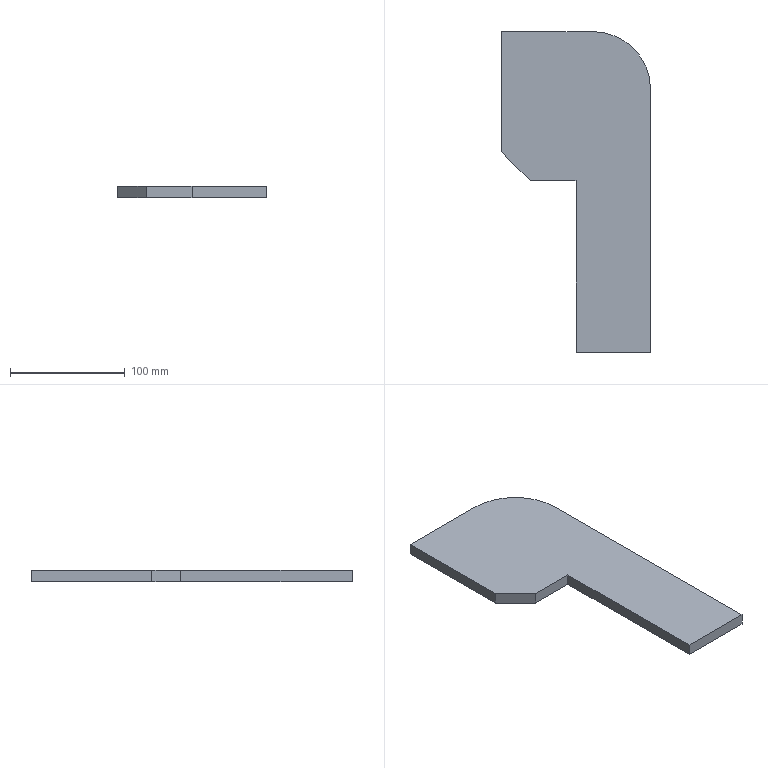Part | SolidWorks | features Extrusion 1 | 1 solid | 10 faces | box 130 x 280 x 10 mm | volume 258010 mm3 | plane 9 | cylinder 1 | commonest cylinder face diameters 100 x1
STEP:
#1=CARTESIAN_POINT('',(80.,280.,-5.));
#2=VERTEX_POINT('',#1);
#3=CARTESIAN_POINT('',(0.,280.,-5.));
#4=VERTEX_POINT('',#3);
#5=CARTESIAN_POINT('',(0.,280.,-5.));
#6=DIRECTION('',(-1.,0.,0.));
#7=VECTOR('',#6,1000.);
#8=LINE('',#5,#7);
#9=EDGE_CURVE('',#2,#4,#8,.T.);
#10=ORIENTED_EDGE('',*,*,#9,.T.);
#11=CARTESIAN_POINT('',(0.,280.,5.));
#12=VERTEX_POINT('',#11);
#13=CARTESIAN_POINT('',(0.,280.,5.));
#14=DIRECTION('',(0.,0.,-1.));
#15=VECTOR('',#14,1000.);
#16=LINE('',#13,#15);
#17=EDGE_CURVE('',#12,#4,#16,.T.);
#18=ORIENTED_EDGE('',*,*,#17,.F.);
#19=CARTESIAN_POINT('',(80.,280.,5.));
#20=VERTEX_POINT('',#19);
#21=CARTESIAN_POINT('',(0.,280.,5.));
#22=DIRECTION('',(-1.,0.,0.));
#23=VECTOR('',#22,1000.);
#24=LINE('',#21,#23);
#25=EDGE_CURVE('',#20,#12,#24,.T.);
#26=ORIENTED_EDGE('',*,*,#25,.F.);
#27=CARTESIAN_POINT('',(80.,280.,5.));
#28=DIRECTION('',(0.,0.,-1.));
#29=VECTOR('',#28,1000.);
#30=LINE('',#27,#29);
#31=EDGE_CURVE('',#20,#2,#30,.T.);
#32=ORIENTED_EDGE('',*,*,#31,.T.);
#33=EDGE_LOOP('',(#10,#18,#26,#32));
#34=FACE_OUTER_BOUND('',#33,.T.);
#35=CARTESIAN_POINT('',(0.,280.,5.));
#36=DIRECTION('',(0.,-1.,0.));
#37=DIRECTION('',(0.,0.,-1.));
#38=AXIS2_PLACEMENT_3D('',#35,#36,#37);
#39=PLANE('',#38);
#40=ADVANCED_FACE('',(#34),#39,.F.);
#41=CARTESIAN_POINT('',(0.,175.,-5.));
#42=VERTEX_POINT('',#41);
#43=CARTESIAN_POINT('',(0.,175.,-5.));
#44=DIRECTION('',(0.,-1.,0.));
#45=VECTOR('',#44,1000.);
#46=LINE('',#43,#45);
#47=EDGE_CURVE('',#4,#42,#46,.T.);
#48=ORIENTED_EDGE('',*,*,#47,.T.);
#49=CARTESIAN_POINT('',(0.,175.,5.));
#50=VERTEX_POINT('',#49);
#51=CARTESIAN_POINT('',(0.,175.,5.));
#52=DIRECTION('',(0.,0.,-1.));
#53=VECTOR('',#52,1000.);
#54=LINE('',#51,#53);
#55=EDGE_CURVE('',#50,#42,#54,.T.);
#56=ORIENTED_EDGE('',*,*,#55,.F.);
#57=CARTESIAN_POINT('',(0.,175.,5.));
#58=DIRECTION('',(0.,-1.,0.));
#59=VECTOR('',#58,1000.);
#60=LINE('',#57,#59);
#61=EDGE_CURVE('',#12,#50,#60,.T.);
#62=ORIENTED_EDGE('',*,*,#61,.F.);
#63=ORIENTED_EDGE('',*,*,#17,.T.);
#64=EDGE_LOOP('',(#48,#56,#62,#63));
#65=FACE_OUTER_BOUND('',#64,.T.);
#66=CARTESIAN_POINT('',(0.,175.,5.));
#67=DIRECTION('',(1.,0.,0.));
#68=DIRECTION('',(0.,0.,-1.));
#69=AXIS2_PLACEMENT_3D('',#66,#67,#68);
#70=PLANE('',#69);
#71=ADVANCED_FACE('',(#65),#70,.F.);
#72=CARTESIAN_POINT('',(25.,150.,-5.));
#73=VERTEX_POINT('',#72);
#74=CARTESIAN_POINT('',(25.,150.,-5.));
#75=DIRECTION('',(0.7071,-0.7071,0.));
#76=VECTOR('',#75,1000.);
#77=LINE('',#74,#76);
#78=EDGE_CURVE('',#42,#73,#77,.T.);
#79=ORIENTED_EDGE('',*,*,#78,.T.);
#80=CARTESIAN_POINT('',(25.,150.,5.));
#81=VERTEX_POINT('',#80);
#82=CARTESIAN_POINT('',(25.,150.,5.));
#83=DIRECTION('',(0.,0.,-1.));
#84=VECTOR('',#83,1000.);
#85=LINE('',#82,#84);
#86=EDGE_CURVE('',#81,#73,#85,.T.);
#87=ORIENTED_EDGE('',*,*,#86,.F.);
#88=CARTESIAN_POINT('',(25.,150.,5.));
#89=DIRECTION('',(0.7071,-0.7071,0.));
#90=VECTOR('',#89,1000.);
#91=LINE('',#88,#90);
#92=EDGE_CURVE('',#50,#81,#91,.T.);
#93=ORIENTED_EDGE('',*,*,#92,.F.);
#94=ORIENTED_EDGE('',*,*,#55,.T.);
#95=EDGE_LOOP('',(#79,#87,#93,#94));
#96=FACE_OUTER_BOUND('',#95,.T.);
#97=CARTESIAN_POINT('',(25.,150.,5.));
#98=DIRECTION('',(0.7071,0.7071,0.));
#99=DIRECTION('',(-0.7071,0.7071,0.));
#100=AXIS2_PLACEMENT_3D('',#97,#98,#99);
#101=PLANE('',#100);
#102=ADVANCED_FACE('',(#96),#101,.F.);
#103=CARTESIAN_POINT('',(65.,150.,-5.));
#104=VERTEX_POINT('',#103);
#105=CARTESIAN_POINT('',(65.,150.,-5.));
#106=DIRECTION('',(1.,0.,0.));
#107=VECTOR('',#106,1000.);
#108=LINE('',#105,#107);
#109=EDGE_CURVE('',#73,#104,#108,.T.);
#110=ORIENTED_EDGE('',*,*,#109,.T.);
#111=CARTESIAN_POINT('',(65.,150.,5.));
#112=VERTEX_POINT('',#111);
#113=CARTESIAN_POINT('',(65.,150.,5.));
#114=DIRECTION('',(0.,0.,-1.));
#115=VECTOR('',#114,1000.);
#116=LINE('',#113,#115);
#117=EDGE_CURVE('',#112,#104,#116,.T.);
#118=ORIENTED_EDGE('',*,*,#117,.F.);
#119=CARTESIAN_POINT('',(65.,150.,5.));
#120=DIRECTION('',(1.,0.,0.));
#121=VECTOR('',#120,1000.);
#122=LINE('',#119,#121);
#123=EDGE_CURVE('',#81,#112,#122,.T.);
#124=ORIENTED_EDGE('',*,*,#123,.F.);
#125=ORIENTED_EDGE('',*,*,#86,.T.);
#126=EDGE_LOOP('',(#110,#118,#124,#125));
#127=FACE_OUTER_BOUND('',#126,.T.);
#128=CARTESIAN_POINT('',(65.,150.,5.));
#129=DIRECTION('',(0.,1.,0.));
#130=DIRECTION('',(-1.,0.,0.));
#131=AXIS2_PLACEMENT_3D('',#128,#129,#130);
#132=PLANE('',#131);
#133=ADVANCED_FACE('',(#127),#132,.F.);
#134=CARTESIAN_POINT('',(65.,0.,-5.));
#135=VERTEX_POINT('',#134);
#136=CARTESIAN_POINT('',(65.,0.,-5.));
#137=DIRECTION('',(0.,-1.,0.));
#138=VECTOR('',#137,1000.);
#139=LINE('',#136,#138);
#140=EDGE_CURVE('',#104,#135,#139,.T.);
#141=ORIENTED_EDGE('',*,*,#140,.T.);
#142=CARTESIAN_POINT('',(65.,0.,5.));
#143=VERTEX_POINT('',#142);
#144=CARTESIAN_POINT('',(65.,0.,5.));
#145=DIRECTION('',(0.,0.,-1.));
#146=VECTOR('',#145,1000.);
#147=LINE('',#144,#146);
#148=EDGE_CURVE('',#143,#135,#147,.T.);
#149=ORIENTED_EDGE('',*,*,#148,.F.);
#150=CARTESIAN_POINT('',(65.,0.,5.));
#151=DIRECTION('',(0.,-1.,0.));
#152=VECTOR('',#151,1000.);
#153=LINE('',#150,#152);
#154=EDGE_CURVE('',#112,#143,#153,.T.);
#155=ORIENTED_EDGE('',*,*,#154,.F.);
#156=ORIENTED_EDGE('',*,*,#117,.T.);
#157=EDGE_LOOP('',(#141,#149,#155,#156));
#158=FACE_OUTER_BOUND('',#157,.T.);
#159=CARTESIAN_POINT('',(65.,0.,5.));
#160=DIRECTION('',(1.,0.,0.));
#161=DIRECTION('',(0.,0.,-1.));
#162=AXIS2_PLACEMENT_3D('',#159,#160,#161);
#163=PLANE('',#162);
#164=ADVANCED_FACE('',(#158),#163,.F.);
#165=CARTESIAN_POINT('',(130.,0.,-5.));
#166=VERTEX_POINT('',#165);
#167=CARTESIAN_POINT('',(130.,0.,-5.));
#168=DIRECTION('',(1.,0.,0.));
#169=VECTOR('',#168,1000.);
#170=LINE('',#167,#169);
#171=EDGE_CURVE('',#135,#166,#170,.T.);
#172=ORIENTED_EDGE('',*,*,#171,.T.);
#173=CARTESIAN_POINT('',(130.,0.,5.));
#174=VERTEX_POINT('',#173);
#175=CARTESIAN_POINT('',(130.,0.,5.));
#176=DIRECTION('',(0.,0.,-1.));
#177=VECTOR('',#176,1000.);
#178=LINE('',#175,#177);
#179=EDGE_CURVE('',#174,#166,#178,.T.);
#180=ORIENTED_EDGE('',*,*,#179,.F.);
#181=CARTESIAN_POINT('',(130.,0.,5.));
#182=DIRECTION('',(1.,0.,0.));
#183=VECTOR('',#182,1000.);
#184=LINE('',#181,#183);
#185=EDGE_CURVE('',#143,#174,#184,.T.);
#186=ORIENTED_EDGE('',*,*,#185,.F.);
#187=ORIENTED_EDGE('',*,*,#148,.T.);
#188=EDGE_LOOP('',(#172,#180,#186,#187));
#189=FACE_OUTER_BOUND('',#188,.T.);
#190=CARTESIAN_POINT('',(130.,0.,5.));
#191=DIRECTION('',(0.,1.,0.));
#192=DIRECTION('',(-1.,0.,0.));
#193=AXIS2_PLACEMENT_3D('',#190,#191,#192);
#194=PLANE('',#193);
#195=ADVANCED_FACE('',(#189),#194,.F.);
#196=CARTESIAN_POINT('',(130.,230.,-5.));
#197=VERTEX_POINT('',#196);
#198=CARTESIAN_POINT('',(130.,230.,-5.));
#199=DIRECTION('',(0.,1.,0.));
#200=VECTOR('',#199,1000.);
#201=LINE('',#198,#200);
#202=EDGE_CURVE('',#166,#197,#201,.T.);
#203=ORIENTED_EDGE('',*,*,#202,.T.);
#204=CARTESIAN_POINT('',(130.,230.,5.));
#205=VERTEX_POINT('',#204);
#206=CARTESIAN_POINT('',(130.,230.,5.));
#207=DIRECTION('',(0.,0.,-1.));
#208=VECTOR('',#207,1000.);
#209=LINE('',#206,#208);
#210=EDGE_CURVE('',#205,#197,#209,.T.);
#211=ORIENTED_EDGE('',*,*,#210,.F.);
#212=CARTESIAN_POINT('',(130.,230.,5.));
#213=DIRECTION('',(0.,1.,0.));
#214=VECTOR('',#213,1000.);
#215=LINE('',#212,#214);
#216=EDGE_CURVE('',#174,#205,#215,.T.);
#217=ORIENTED_EDGE('',*,*,#216,.F.);
#218=ORIENTED_EDGE('',*,*,#179,.T.);
#219=EDGE_LOOP('',(#203,#211,#217,#218));
#220=FACE_OUTER_BOUND('',#219,.T.);
#221=CARTESIAN_POINT('',(130.,230.,5.));
#222=DIRECTION('',(-1.,0.,0.));
#223=DIRECTION('',(0.,0.,1.));
#224=AXIS2_PLACEMENT_3D('',#221,#222,#223);
#225=PLANE('',#224);
#226=ADVANCED_FACE('',(#220),#225,.F.);
#227=CARTESIAN_POINT('',(80.,230.,-5.));
#228=DIRECTION('',(0.,0.,1.));
#229=DIRECTION('',(-1.,0.,0.));
#230=AXIS2_PLACEMENT_3D('',#227,#228,#229);
#231=CIRCLE('',#230,50.);
#232=EDGE_CURVE('',#197,#2,#231,.T.);
#233=ORIENTED_EDGE('',*,*,#232,.T.);
#234=ORIENTED_EDGE('',*,*,#31,.F.);
#235=CARTESIAN_POINT('',(80.,230.,5.));
#236=DIRECTION('',(0.,0.,1.));
#237=DIRECTION('',(-1.,0.,0.));
#238=AXIS2_PLACEMENT_3D('',#235,#236,#237);
#239=CIRCLE('',#238,50.);
#240=EDGE_CURVE('',#205,#20,#239,.T.);
#241=ORIENTED_EDGE('',*,*,#240,.F.);
#242=ORIENTED_EDGE('',*,*,#210,.T.);
#243=EDGE_LOOP('',(#233,#234,#241,#242));
#244=FACE_OUTER_BOUND('',#243,.T.);
#245=CARTESIAN_POINT('',(80.,230.,5.));
#246=DIRECTION('',(0.,0.,-1.));
#247=DIRECTION('',(-1.,0.,0.));
#248=AXIS2_PLACEMENT_3D('',#245,#246,#247);
#249=CYLINDRICAL_SURFACE('',#248,50.);
#250=ADVANCED_FACE('',(#244),#249,.T.);
#251=ORIENTED_EDGE('',*,*,#25,.T.);
#252=ORIENTED_EDGE('',*,*,#61,.T.);
#253=ORIENTED_EDGE('',*,*,#92,.T.);
#254=ORIENTED_EDGE('',*,*,#123,.T.);
#255=ORIENTED_EDGE('',*,*,#154,.T.);
#256=ORIENTED_EDGE('',*,*,#185,.T.);
#257=ORIENTED_EDGE('',*,*,#216,.T.);
#258=ORIENTED_EDGE('',*,*,#240,.T.);
#259=EDGE_LOOP('',(#251,#252,#253,#254,#255,#256,#257,#258));
#260=FACE_OUTER_BOUND('',#259,.T.);
#261=CARTESIAN_POINT('',(80.,230.,5.));
#262=DIRECTION('',(0.,0.,-1.));
#263=DIRECTION('',(-1.,0.,0.));
#264=AXIS2_PLACEMENT_3D('',#261,#262,#263);
#265=PLANE('',#264);
#266=ADVANCED_FACE('',(#260),#265,.F.);
#267=ORIENTED_EDGE('',*,*,#9,.F.);
#268=ORIENTED_EDGE('',*,*,#232,.F.);
#269=ORIENTED_EDGE('',*,*,#202,.F.);
#270=ORIENTED_EDGE('',*,*,#171,.F.);
#271=ORIENTED_EDGE('',*,*,#140,.F.);
#272=ORIENTED_EDGE('',*,*,#109,.F.);
#273=ORIENTED_EDGE('',*,*,#78,.F.);
#274=ORIENTED_EDGE('',*,*,#47,.F.);
#275=EDGE_LOOP('',(#267,#268,#269,#270,#271,#272,#273,#274));
#276=FACE_OUTER_BOUND('',#275,.T.);
#277=CARTESIAN_POINT('',(80.,230.,-5.));
#278=DIRECTION('',(0.,0.,-1.));
#279=DIRECTION('',(-1.,0.,0.));
#280=AXIS2_PLACEMENT_3D('',#277,#278,#279);
#281=PLANE('',#280);
#282=ADVANCED_FACE('',(#276),#281,.T.);
#283=CLOSED_SHELL('',(#40,#71,#102,#133,#164,#195,#226,#250,#266,#282));
#284=MANIFOLD_SOLID_BREP('',#283);
#285=CARTESIAN_POINT('',(0.,0.,0.));
#286=DIRECTION('',(0.,0.,1.));
#287=DIRECTION('',(1.,0.,0.));
#288=AXIS2_PLACEMENT_3D('',#285,#286,#287);
#289=(LENGTH_UNIT()NAMED_UNIT(*)SI_UNIT(.MILLI.,.METRE.));
#290=UNCERTAINTY_MEASURE_WITH_UNIT(LENGTH_MEASURE(0.00001),#289,'','');
#291=(NAMED_UNIT(*)PLANE_ANGLE_UNIT()SI_UNIT($,.RADIAN.));
#292=(NAMED_UNIT(*)SI_UNIT($,.STERADIAN.)SOLID_ANGLE_UNIT());
#293=(GEOMETRIC_REPRESENTATION_CONTEXT(3)GLOBAL_UNCERTAINTY_ASSIGNED_CONTEXT((#290))GLOBAL_UNIT_ASSIGNED_CONTEXT((#289,#291,#292))REPRESENTATION_CONTEXT('',''));
#294=ADVANCED_BREP_SHAPE_REPRESENTATION('',(#284,#288),#293);